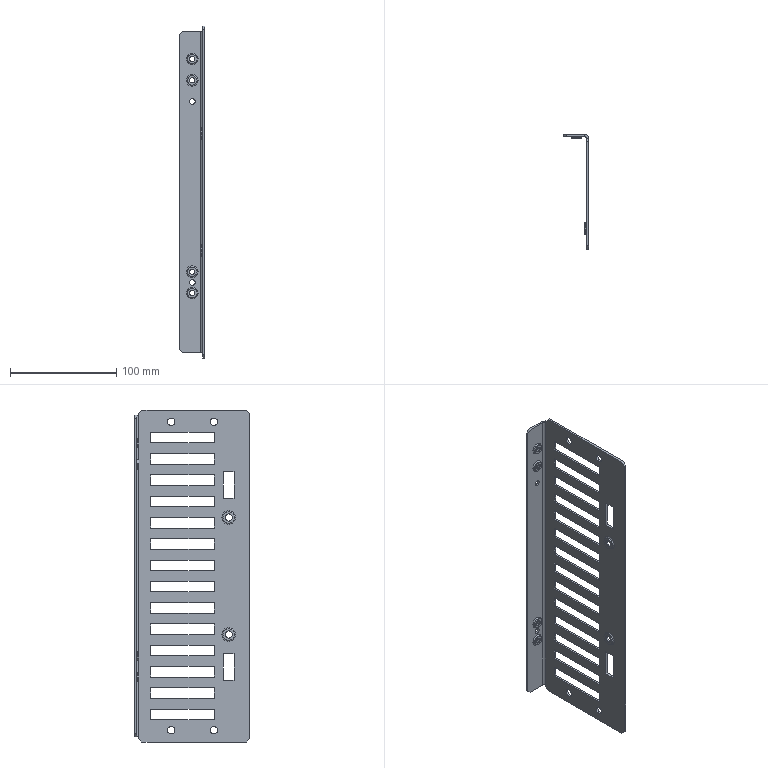Part | STEP file | 64586742 | 1 solid | 152 faces | box 24 x 108 x 312 mm | volume 61627 mm3 | plane 90 | cylinder 38 | torus 24 | commonest cylinder face diameters 5 x8 7 x8 9 x8 5.4 x4 6.8 x4 10.8 x4